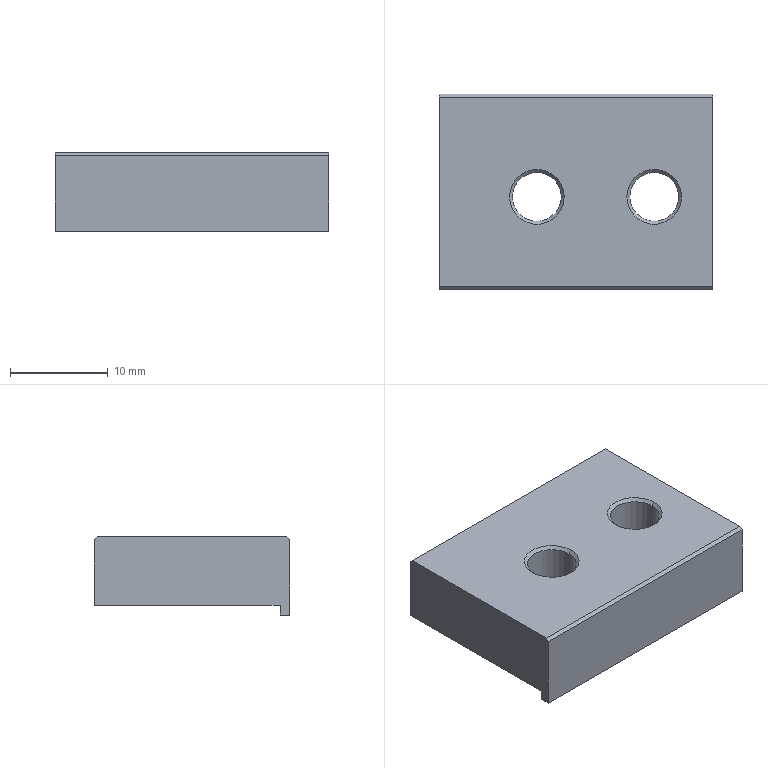Part | NX | 1 solid | 22 faces | box 28 x 20 x 8 mm | volume 3668 mm3 | plane 10 | cone 8 | cylinder 4 | commonest cylinder face diameters 5 x4
STEP:
#1=CARTESIAN_POINT('',(28.,0.7,7.));
#2=VERTEX_POINT('',#1);
#3=CARTESIAN_POINT('',(0.,0.7,7.));
#4=VERTEX_POINT('',#3);
#5=CARTESIAN_POINT('',(0.,0.7,7.));
#6=DIRECTION('',(-1.,0.,0.));
#7=VECTOR('',#6,1000.);
#8=LINE('',#5,#7);
#9=EDGE_CURVE('',#2,#4,#8,.T.);
#10=ORIENTED_EDGE('',*,*,#9,.T.);
#11=CARTESIAN_POINT('',(0.,-18.7,7.));
#12=VERTEX_POINT('',#11);
#13=CARTESIAN_POINT('',(0.,0.,7.));
#14=DIRECTION('',(0.,1.,0.));
#15=VECTOR('',#14,1000.);
#16=LINE('',#13,#15);
#17=EDGE_CURVE('',#12,#4,#16,.T.);
#18=ORIENTED_EDGE('',*,*,#17,.F.);
#19=CARTESIAN_POINT('',(28.,-18.7,7.));
#20=VERTEX_POINT('',#19);
#21=CARTESIAN_POINT('',(0.,-18.7,7.));
#22=DIRECTION('',(1.,0.,0.));
#23=VECTOR('',#22,1000.);
#24=LINE('',#21,#23);
#25=EDGE_CURVE('',#12,#20,#24,.T.);
#26=ORIENTED_EDGE('',*,*,#25,.T.);
#27=CARTESIAN_POINT('',(28.,0.,7.));
#28=DIRECTION('',(0.,-1.,0.));
#29=VECTOR('',#28,1000.);
#30=LINE('',#27,#29);
#31=EDGE_CURVE('',#2,#20,#30,.T.);
#32=ORIENTED_EDGE('',*,*,#31,.F.);
#33=EDGE_LOOP('',(#10,#18,#26,#32));
#34=FACE_BOUND('',#33,.T.);
#35=CARTESIAN_POINT('',(12.8,-9.5,7.));
#36=VERTEX_POINT('',#35);
#37=CARTESIAN_POINT('',(7.2,-9.5,7.));
#38=VERTEX_POINT('',#37);
#39=CARTESIAN_POINT('',(10.,-9.5,7.));
#40=DIRECTION('',(0.,0.,1.));
#41=DIRECTION('',(1.,0.,0.));
#42=AXIS2_PLACEMENT_3D('',#39,#40,#41);
#43=CIRCLE('',#42,2.8);
#44=EDGE_CURVE('',#36,#38,#43,.T.);
#45=ORIENTED_EDGE('',*,*,#44,.F.);
#46=CARTESIAN_POINT('',(10.,-9.5,7.));
#47=DIRECTION('',(0.,0.,1.));
#48=DIRECTION('',(1.,0.,0.));
#49=AXIS2_PLACEMENT_3D('',#46,#47,#48);
#50=CIRCLE('',#49,2.8);
#51=EDGE_CURVE('',#38,#36,#50,.T.);
#52=ORIENTED_EDGE('',*,*,#51,.F.);
#53=EDGE_LOOP('',(#45,#52));
#54=FACE_BOUND('',#53,.T.);
#55=CARTESIAN_POINT('',(19.2,-9.5,7.));
#56=VERTEX_POINT('',#55);
#57=CARTESIAN_POINT('',(24.8,-9.5,7.));
#58=VERTEX_POINT('',#57);
#59=CARTESIAN_POINT('',(22.,-9.5,7.));
#60=DIRECTION('',(0.,0.,1.));
#61=DIRECTION('',(1.,0.,0.));
#62=AXIS2_PLACEMENT_3D('',#59,#60,#61);
#63=CIRCLE('',#62,2.8);
#64=EDGE_CURVE('',#56,#58,#63,.T.);
#65=ORIENTED_EDGE('',*,*,#64,.F.);
#66=CARTESIAN_POINT('',(22.,-9.5,7.));
#67=DIRECTION('',(0.,0.,1.));
#68=DIRECTION('',(1.,0.,0.));
#69=AXIS2_PLACEMENT_3D('',#66,#67,#68);
#70=CIRCLE('',#69,2.8);
#71=EDGE_CURVE('',#58,#56,#70,.T.);
#72=ORIENTED_EDGE('',*,*,#71,.F.);
#73=EDGE_LOOP('',(#65,#72));
#74=FACE_BOUND('',#73,.T.);
#75=CARTESIAN_POINT('',(0.,0.,7.));
#76=DIRECTION('',(0.,0.,1.));
#77=DIRECTION('',(1.,0.,0.));
#78=AXIS2_PLACEMENT_3D('',#75,#76,#77);
#79=PLANE('',#78);
#80=ADVANCED_FACE('',(#34,#54,#74),#79,.T.);
#81=CARTESIAN_POINT('',(28.,1.,0.));
#82=VERTEX_POINT('',#81);
#83=CARTESIAN_POINT('',(28.,1.,6.7));
#84=VERTEX_POINT('',#83);
#85=CARTESIAN_POINT('',(28.,1.,0.));
#86=DIRECTION('',(0.,0.,1.));
#87=VECTOR('',#86,1000.);
#88=LINE('',#85,#87);
#89=EDGE_CURVE('',#82,#84,#88,.T.);
#90=ORIENTED_EDGE('',*,*,#89,.T.);
#91=CARTESIAN_POINT('',(28.,0.,7.7));
#92=DIRECTION('',(0.,-0.7071,0.7071));
#93=VECTOR('',#92,1000.);
#94=LINE('',#91,#93);
#95=EDGE_CURVE('',#84,#2,#94,.T.);
#96=ORIENTED_EDGE('',*,*,#95,.T.);
#97=ORIENTED_EDGE('',*,*,#31,.T.);
#98=CARTESIAN_POINT('',(28.,-19.,6.7));
#99=VERTEX_POINT('',#98);
#100=CARTESIAN_POINT('',(28.,0.,25.7));
#101=DIRECTION('',(0.,-0.7071,-0.7071));
#102=VECTOR('',#101,1000.);
#103=LINE('',#100,#102);
#104=EDGE_CURVE('',#20,#99,#103,.T.);
#105=ORIENTED_EDGE('',*,*,#104,.T.);
#106=CARTESIAN_POINT('',(28.,-19.,-1.));
#107=VERTEX_POINT('',#106);
#108=CARTESIAN_POINT('',(28.,-19.,0.));
#109=DIRECTION('',(0.,0.,-1.));
#110=VECTOR('',#109,1000.);
#111=LINE('',#108,#110);
#112=EDGE_CURVE('',#99,#107,#111,.T.);
#113=ORIENTED_EDGE('',*,*,#112,.T.);
#114=CARTESIAN_POINT('',(28.,-18.,-1.));
#115=VERTEX_POINT('',#114);
#116=CARTESIAN_POINT('',(28.,0.,-1.));
#117=DIRECTION('',(0.,1.,0.));
#118=VECTOR('',#117,1000.);
#119=LINE('',#116,#118);
#120=EDGE_CURVE('',#107,#115,#119,.T.);
#121=ORIENTED_EDGE('',*,*,#120,.T.);
#122=CARTESIAN_POINT('',(28.,-18.,0.));
#123=VERTEX_POINT('',#122);
#124=CARTESIAN_POINT('',(28.,-18.,0.));
#125=DIRECTION('',(0.,0.,-1.));
#126=VECTOR('',#125,1000.);
#127=LINE('',#124,#126);
#128=EDGE_CURVE('',#123,#115,#127,.T.);
#129=ORIENTED_EDGE('',*,*,#128,.F.);
#130=CARTESIAN_POINT('',(28.,0.,0.));
#131=DIRECTION('',(0.,-1.,0.));
#132=VECTOR('',#131,1000.);
#133=LINE('',#130,#132);
#134=EDGE_CURVE('',#82,#123,#133,.T.);
#135=ORIENTED_EDGE('',*,*,#134,.F.);
#136=EDGE_LOOP('',(#90,#96,#97,#105,#113,#121,#129,#135));
#137=FACE_BOUND('',#136,.T.);
#138=CARTESIAN_POINT('',(28.,-18.,0.));
#139=DIRECTION('',(1.,0.,0.));
#140=DIRECTION('',(0.,1.,0.));
#141=AXIS2_PLACEMENT_3D('',#138,#139,#140);
#142=PLANE('',#141);
#143=ADVANCED_FACE('',(#137),#142,.T.);
#144=CARTESIAN_POINT('',(0.,-18.,0.));
#145=VERTEX_POINT('',#144);
#146=CARTESIAN_POINT('',(0.,-18.,0.));
#147=DIRECTION('',(-1.,0.,0.));
#148=VECTOR('',#147,1000.);
#149=LINE('',#146,#148);
#150=EDGE_CURVE('',#123,#145,#149,.T.);
#151=ORIENTED_EDGE('',*,*,#150,.F.);
#152=ORIENTED_EDGE('',*,*,#128,.T.);
#153=CARTESIAN_POINT('',(0.,-18.,-1.));
#154=VERTEX_POINT('',#153);
#155=CARTESIAN_POINT('',(0.,-18.,-1.));
#156=DIRECTION('',(1.,0.,0.));
#157=VECTOR('',#156,1000.);
#158=LINE('',#155,#157);
#159=EDGE_CURVE('',#154,#115,#158,.T.);
#160=ORIENTED_EDGE('',*,*,#159,.F.);
#161=CARTESIAN_POINT('',(0.,-18.,0.));
#162=DIRECTION('',(0.,0.,1.));
#163=VECTOR('',#162,1000.);
#164=LINE('',#161,#163);
#165=EDGE_CURVE('',#154,#145,#164,.T.);
#166=ORIENTED_EDGE('',*,*,#165,.T.);
#167=EDGE_LOOP('',(#151,#152,#160,#166));
#168=FACE_BOUND('',#167,.T.);
#169=CARTESIAN_POINT('',(0.,-18.,0.));
#170=DIRECTION('',(0.,-1.,0.));
#171=DIRECTION('',(0.,0.,-1.));
#172=AXIS2_PLACEMENT_3D('',#169,#170,#171);
#173=PLANE('',#172);
#174=ADVANCED_FACE('',(#168),#173,.F.);
#175=CARTESIAN_POINT('',(0.,1.,0.));
#176=VERTEX_POINT('',#175);
#177=CARTESIAN_POINT('',(0.,0.,0.));
#178=DIRECTION('',(0.,1.,0.));
#179=VECTOR('',#178,1000.);
#180=LINE('',#177,#179);
#181=EDGE_CURVE('',#145,#176,#180,.T.);
#182=ORIENTED_EDGE('',*,*,#181,.F.);
#183=ORIENTED_EDGE('',*,*,#165,.F.);
#184=CARTESIAN_POINT('',(0.,-19.,-1.));
#185=VERTEX_POINT('',#184);
#186=CARTESIAN_POINT('',(0.,0.,-1.));
#187=DIRECTION('',(0.,-1.,0.));
#188=VECTOR('',#187,1000.);
#189=LINE('',#186,#188);
#190=EDGE_CURVE('',#154,#185,#189,.T.);
#191=ORIENTED_EDGE('',*,*,#190,.T.);
#192=CARTESIAN_POINT('',(0.,-19.,6.7));
#193=VERTEX_POINT('',#192);
#194=CARTESIAN_POINT('',(0.,-19.,0.));
#195=DIRECTION('',(0.,0.,1.));
#196=VECTOR('',#195,1000.);
#197=LINE('',#194,#196);
#198=EDGE_CURVE('',#185,#193,#197,.T.);
#199=ORIENTED_EDGE('',*,*,#198,.T.);
#200=CARTESIAN_POINT('',(0.,0.,25.7));
#201=DIRECTION('',(0.,0.7071,0.7071));
#202=VECTOR('',#201,1000.);
#203=LINE('',#200,#202);
#204=EDGE_CURVE('',#193,#12,#203,.T.);
#205=ORIENTED_EDGE('',*,*,#204,.T.);
#206=ORIENTED_EDGE('',*,*,#17,.T.);
#207=CARTESIAN_POINT('',(0.,1.,6.7));
#208=VERTEX_POINT('',#207);
#209=CARTESIAN_POINT('',(0.,0.,7.7));
#210=DIRECTION('',(0.,0.7071,-0.7071));
#211=VECTOR('',#210,1000.);
#212=LINE('',#209,#211);
#213=EDGE_CURVE('',#4,#208,#212,.T.);
#214=ORIENTED_EDGE('',*,*,#213,.T.);
#215=CARTESIAN_POINT('',(0.,1.,0.));
#216=DIRECTION('',(0.,0.,-1.));
#217=VECTOR('',#216,1000.);
#218=LINE('',#215,#217);
#219=EDGE_CURVE('',#208,#176,#218,.T.);
#220=ORIENTED_EDGE('',*,*,#219,.T.);
#221=EDGE_LOOP('',(#182,#183,#191,#199,#205,#206,#214,#220));
#222=FACE_BOUND('',#221,.T.);
#223=CARTESIAN_POINT('',(0.,0.,0.));
#224=DIRECTION('',(-1.,0.,0.));
#225=DIRECTION('',(0.,0.,1.));
#226=AXIS2_PLACEMENT_3D('',#223,#224,#225);
#227=PLANE('',#226);
#228=ADVANCED_FACE('',(#222),#227,.T.);
#229=CARTESIAN_POINT('',(0.,1.,0.));
#230=DIRECTION('',(1.,0.,0.));
#231=VECTOR('',#230,1000.);
#232=LINE('',#229,#231);
#233=EDGE_CURVE('',#176,#82,#232,.T.);
#234=ORIENTED_EDGE('',*,*,#233,.T.);
#235=ORIENTED_EDGE('',*,*,#134,.T.);
#236=ORIENTED_EDGE('',*,*,#150,.T.);
#237=ORIENTED_EDGE('',*,*,#181,.T.);
#238=EDGE_LOOP('',(#234,#235,#236,#237));
#239=FACE_BOUND('',#238,.T.);
#240=CARTESIAN_POINT('',(7.2,-9.5,0.));
#241=VERTEX_POINT('',#240);
#242=CARTESIAN_POINT('',(12.8,-9.5,0.));
#243=VERTEX_POINT('',#242);
#244=CARTESIAN_POINT('',(10.,-9.5,0.));
#245=DIRECTION('',(0.,0.,-1.));
#246=DIRECTION('',(-1.,0.,0.));
#247=AXIS2_PLACEMENT_3D('',#244,#245,#246);
#248=CIRCLE('',#247,2.8);
#249=EDGE_CURVE('',#241,#243,#248,.T.);
#250=ORIENTED_EDGE('',*,*,#249,.F.);
#251=CARTESIAN_POINT('',(10.,-9.5,0.));
#252=DIRECTION('',(0.,0.,-1.));
#253=DIRECTION('',(-1.,0.,0.));
#254=AXIS2_PLACEMENT_3D('',#251,#252,#253);
#255=CIRCLE('',#254,2.8);
#256=EDGE_CURVE('',#243,#241,#255,.T.);
#257=ORIENTED_EDGE('',*,*,#256,.F.);
#258=EDGE_LOOP('',(#250,#257));
#259=FACE_BOUND('',#258,.T.);
#260=CARTESIAN_POINT('',(19.2,-9.5,0.));
#261=VERTEX_POINT('',#260);
#262=CARTESIAN_POINT('',(24.8,-9.5,0.));
#263=VERTEX_POINT('',#262);
#264=CARTESIAN_POINT('',(22.,-9.5,0.));
#265=DIRECTION('',(0.,0.,-1.));
#266=DIRECTION('',(-1.,0.,0.));
#267=AXIS2_PLACEMENT_3D('',#264,#265,#266);
#268=CIRCLE('',#267,2.8);
#269=EDGE_CURVE('',#261,#263,#268,.T.);
#270=ORIENTED_EDGE('',*,*,#269,.F.);
#271=CARTESIAN_POINT('',(22.,-9.5,0.));
#272=DIRECTION('',(0.,0.,-1.));
#273=DIRECTION('',(-1.,0.,0.));
#274=AXIS2_PLACEMENT_3D('',#271,#272,#273);
#275=CIRCLE('',#274,2.8);
#276=EDGE_CURVE('',#263,#261,#275,.T.);
#277=ORIENTED_EDGE('',*,*,#276,.F.);
#278=EDGE_LOOP('',(#270,#277));
#279=FACE_BOUND('',#278,.T.);
#280=CARTESIAN_POINT('',(0.,0.,0.));
#281=DIRECTION('',(0.,0.,1.));
#282=DIRECTION('',(1.,0.,0.));
#283=AXIS2_PLACEMENT_3D('',#280,#281,#282);
#284=PLANE('',#283);
#285=ADVANCED_FACE('',(#239,#259,#279),#284,.F.);
#286=CARTESIAN_POINT('',(0.,-19.,6.7));
#287=DIRECTION('',(1.,0.,0.));
#288=VECTOR('',#287,1000.);
#289=LINE('',#286,#288);
#290=EDGE_CURVE('',#193,#99,#289,.T.);
#291=ORIENTED_EDGE('',*,*,#290,.F.);
#292=ORIENTED_EDGE('',*,*,#198,.F.);
#293=CARTESIAN_POINT('',(0.,-19.,-1.));
#294=DIRECTION('',(-1.,0.,0.));
#295=VECTOR('',#294,1000.);
#296=LINE('',#293,#295);
#297=EDGE_CURVE('',#107,#185,#296,.T.);
#298=ORIENTED_EDGE('',*,*,#297,.F.);
#299=ORIENTED_EDGE('',*,*,#112,.F.);
#300=EDGE_LOOP('',(#291,#292,#298,#299));
#301=FACE_BOUND('',#300,.T.);
#302=CARTESIAN_POINT('',(0.,-19.,0.));
#303=DIRECTION('',(0.,-1.,0.));
#304=DIRECTION('',(0.,0.,-1.));
#305=AXIS2_PLACEMENT_3D('',#302,#303,#304);
#306=PLANE('',#305);
#307=ADVANCED_FACE('',(#301),#306,.T.);
#308=ORIENTED_EDGE('',*,*,#159,.T.);
#309=ORIENTED_EDGE('',*,*,#120,.F.);
#310=ORIENTED_EDGE('',*,*,#297,.T.);
#311=ORIENTED_EDGE('',*,*,#190,.F.);
#312=EDGE_LOOP('',(#308,#309,#310,#311));
#313=FACE_BOUND('',#312,.T.);
#314=CARTESIAN_POINT('',(0.,-18.,-1.));
#315=DIRECTION('',(0.,0.,-1.));
#316=DIRECTION('',(0.,-1.,0.));
#317=AXIS2_PLACEMENT_3D('',#314,#315,#316);
#318=PLANE('',#317);
#319=ADVANCED_FACE('',(#313),#318,.T.);
#320=ORIENTED_EDGE('',*,*,#233,.F.);
#321=ORIENTED_EDGE('',*,*,#219,.F.);
#322=CARTESIAN_POINT('',(0.,1.,6.7));
#323=DIRECTION('',(1.,0.,0.));
#324=VECTOR('',#323,1000.);
#325=LINE('',#322,#324);
#326=EDGE_CURVE('',#208,#84,#325,.T.);
#327=ORIENTED_EDGE('',*,*,#326,.T.);
#328=ORIENTED_EDGE('',*,*,#89,.F.);
#329=EDGE_LOOP('',(#320,#321,#327,#328));
#330=FACE_BOUND('',#329,.T.);
#331=CARTESIAN_POINT('',(28.,1.,0.));
#332=DIRECTION('',(0.,1.,0.));
#333=DIRECTION('',(1.,0.,0.));
#334=AXIS2_PLACEMENT_3D('',#331,#332,#333);
#335=PLANE('',#334);
#336=ADVANCED_FACE('',(#330),#335,.T.);
#337=CARTESIAN_POINT('',(12.5,-9.5,0.3));
#338=VERTEX_POINT('',#337);
#339=CARTESIAN_POINT('',(7.5,-9.5,0.3));
#340=VERTEX_POINT('',#339);
#341=CARTESIAN_POINT('',(10.,-9.5,0.3));
#342=DIRECTION('',(0.,0.,-1.));
#343=DIRECTION('',(-1.,0.,0.));
#344=AXIS2_PLACEMENT_3D('',#341,#342,#343);
#345=CIRCLE('',#344,2.5);
#346=EDGE_CURVE('',#338,#340,#345,.T.);
#347=ORIENTED_EDGE('',*,*,#346,.T.);
#348=CARTESIAN_POINT('',(7.5,-9.5,6.7));
#349=VERTEX_POINT('',#348);
#350=CARTESIAN_POINT('',(7.5,-9.5,7.));
#351=DIRECTION('',(0.,0.,-1.));
#352=VECTOR('',#351,1000.);
#353=LINE('',#350,#352);
#354=EDGE_CURVE('',#340,#349,#353,.F.);
#355=ORIENTED_EDGE('',*,*,#354,.T.);
#356=CARTESIAN_POINT('',(12.5,-9.5,6.7));
#357=VERTEX_POINT('',#356);
#358=CARTESIAN_POINT('',(10.,-9.5,6.7));
#359=DIRECTION('',(0.,0.,1.));
#360=DIRECTION('',(1.,0.,0.));
#361=AXIS2_PLACEMENT_3D('',#358,#359,#360);
#362=CIRCLE('',#361,2.5);
#363=EDGE_CURVE('',#349,#357,#362,.T.);
#364=ORIENTED_EDGE('',*,*,#363,.T.);
#365=CARTESIAN_POINT('',(12.5,-9.5,7.));
#366=DIRECTION('',(0.,0.,-1.));
#367=VECTOR('',#366,1000.);
#368=LINE('',#365,#367);
#369=EDGE_CURVE('',#338,#357,#368,.F.);
#370=ORIENTED_EDGE('',*,*,#369,.F.);
#371=EDGE_LOOP('',(#347,#355,#364,#370));
#372=FACE_BOUND('',#371,.T.);
#373=CARTESIAN_POINT('',(10.,-9.5,7.));
#374=DIRECTION('',(0.,0.,-1.));
#375=DIRECTION('',(-1.,0.,0.));
#376=AXIS2_PLACEMENT_3D('',#373,#374,#375);
#377=CYLINDRICAL_SURFACE('',#376,2.5);
#378=ADVANCED_FACE('',(#372),#377,.F.);
#379=CARTESIAN_POINT('',(19.5,-9.5,6.7));
#380=VERTEX_POINT('',#379);
#381=CARTESIAN_POINT('',(24.5,-9.5,6.7));
#382=VERTEX_POINT('',#381);
#383=CARTESIAN_POINT('',(22.,-9.5,6.7));
#384=DIRECTION('',(0.,0.,1.));
#385=DIRECTION('',(1.,0.,0.));
#386=AXIS2_PLACEMENT_3D('',#383,#384,#385);
#387=CIRCLE('',#386,2.5);
#388=EDGE_CURVE('',#380,#382,#387,.T.);
#389=ORIENTED_EDGE('',*,*,#388,.T.);
#390=CARTESIAN_POINT('',(24.5,-9.5,0.3));
#391=VERTEX_POINT('',#390);
#392=CARTESIAN_POINT('',(24.5,-9.5,7.));
#393=DIRECTION('',(0.,0.,-1.));
#394=VECTOR('',#393,1000.);
#395=LINE('',#392,#394);
#396=EDGE_CURVE('',#382,#391,#395,.T.);
#397=ORIENTED_EDGE('',*,*,#396,.T.);
#398=CARTESIAN_POINT('',(19.5,-9.5,0.3));
#399=VERTEX_POINT('',#398);
#400=CARTESIAN_POINT('',(22.,-9.5,0.3));
#401=DIRECTION('',(0.,0.,-1.));
#402=DIRECTION('',(-1.,0.,0.));
#403=AXIS2_PLACEMENT_3D('',#400,#401,#402);
#404=CIRCLE('',#403,2.5);
#405=EDGE_CURVE('',#391,#399,#404,.T.);
#406=ORIENTED_EDGE('',*,*,#405,.T.);
#407=CARTESIAN_POINT('',(19.5,-9.5,7.));
#408=DIRECTION('',(0.,0.,-1.));
#409=VECTOR('',#408,1000.);
#410=LINE('',#407,#409);
#411=EDGE_CURVE('',#380,#399,#410,.T.);
#412=ORIENTED_EDGE('',*,*,#411,.F.);
#413=EDGE_LOOP('',(#389,#397,#406,#412));
#414=FACE_BOUND('',#413,.T.);
#415=CARTESIAN_POINT('',(22.,-9.5,7.));
#416=DIRECTION('',(0.,0.,-1.));
#417=DIRECTION('',(-1.,0.,0.));
#418=AXIS2_PLACEMENT_3D('',#415,#416,#417);
#419=CYLINDRICAL_SURFACE('',#418,2.5);
#420=ADVANCED_FACE('',(#414),#419,.F.);
#421=ORIENTED_EDGE('',*,*,#25,.F.);
#422=ORIENTED_EDGE('',*,*,#204,.F.);
#423=ORIENTED_EDGE('',*,*,#290,.T.);
#424=ORIENTED_EDGE('',*,*,#104,.F.);
#425=EDGE_LOOP('',(#421,#422,#423,#424));
#426=FACE_BOUND('',#425,.T.);
#427=CARTESIAN_POINT('',(14.,-18.85,6.85));
#428=DIRECTION('',(0.,-0.7071,0.7071));
#429=DIRECTION('',(-1.,0.,0.));
#430=AXIS2_PLACEMENT_3D('',#427,#428,#429);
#431=PLANE('',#430);
#432=ADVANCED_FACE('',(#426),#431,.T.);
#433=CARTESIAN_POINT('',(22.,-9.5,0.3));
#434=DIRECTION('',(0.,0.,-1.));
#435=DIRECTION('',(-1.,0.,0.));
#436=AXIS2_PLACEMENT_3D('',#433,#434,#435);
#437=CIRCLE('',#436,2.5);
#438=EDGE_CURVE('',#399,#391,#437,.T.);
#439=ORIENTED_EDGE('',*,*,#438,.F.);
#440=CARTESIAN_POINT('',(19.2,-9.5,0.));
#441=DIRECTION('',(-0.7071,0.,-0.7071));
#442=VECTOR('',#441,1000.);
#443=LINE('',#440,#442);
#444=EDGE_CURVE('',#261,#399,#443,.F.);
#445=ORIENTED_EDGE('',*,*,#444,.F.);
#446=ORIENTED_EDGE('',*,*,#269,.T.);
#447=CARTESIAN_POINT('',(24.8,-9.5,0.));
#448=DIRECTION('',(0.7071,0.,-0.7071));
#449=VECTOR('',#448,1000.);
#450=LINE('',#447,#449);
#451=EDGE_CURVE('',#263,#391,#450,.F.);
#452=ORIENTED_EDGE('',*,*,#451,.T.);
#453=EDGE_LOOP('',(#439,#445,#446,#452));
#454=FACE_BOUND('',#453,.T.);
#455=CARTESIAN_POINT('',(22.,-9.5,0.));
#456=DIRECTION('',(0.,0.,-1.));
#457=DIRECTION('',(-1.,0.,0.));
#458=AXIS2_PLACEMENT_3D('',#455,#456,#457);
#459=CONICAL_SURFACE('',#458,2.8,0.7854);
#460=ADVANCED_FACE('',(#454),#459,.F.);
#461=ORIENTED_EDGE('',*,*,#346,.F.);
#462=CARTESIAN_POINT('',(12.8,-9.5,0.));
#463=DIRECTION('',(0.7071,0.,-0.7071));
#464=VECTOR('',#463,1000.);
#465=LINE('',#462,#464);
#466=EDGE_CURVE('',#338,#243,#465,.T.);
#467=ORIENTED_EDGE('',*,*,#466,.T.);
#468=ORIENTED_EDGE('',*,*,#256,.T.);
#469=CARTESIAN_POINT('',(7.2,-9.5,0.));
#470=DIRECTION('',(-0.7071,0.,-0.7071));
#471=VECTOR('',#470,1000.);
#472=LINE('',#469,#471);
#473=EDGE_CURVE('',#340,#241,#472,.T.);
#474=ORIENTED_EDGE('',*,*,#473,.F.);
#475=EDGE_LOOP('',(#461,#467,#468,#474));
#476=FACE_BOUND('',#475,.T.);
#477=CARTESIAN_POINT('',(10.,-9.5,0.));
#478=DIRECTION('',(0.,0.,-1.));
#479=DIRECTION('',(-1.,0.,0.));
#480=AXIS2_PLACEMENT_3D('',#477,#478,#479);
#481=CONICAL_SURFACE('',#480,2.8,0.7854);
#482=ADVANCED_FACE('',(#476),#481,.F.);
#483=ORIENTED_EDGE('',*,*,#363,.F.);
#484=CARTESIAN_POINT('',(7.2,-9.5,7.));
#485=DIRECTION('',(-0.7071,0.,0.7071));
#486=VECTOR('',#485,1000.);
#487=LINE('',#484,#486);
#488=EDGE_CURVE('',#38,#349,#487,.F.);
#489=ORIENTED_EDGE('',*,*,#488,.F.);
#490=ORIENTED_EDGE('',*,*,#51,.T.);
#491=CARTESIAN_POINT('',(12.8,-9.5,7.));
#492=DIRECTION('',(0.7071,0.,0.7071));
#493=VECTOR('',#492,1000.);
#494=LINE('',#491,#493);
#495=EDGE_CURVE('',#36,#357,#494,.F.);
#496=ORIENTED_EDGE('',*,*,#495,.T.);
#497=EDGE_LOOP('',(#483,#489,#490,#496));
#498=FACE_BOUND('',#497,.T.);
#499=CARTESIAN_POINT('',(10.,-9.5,7.));
#500=DIRECTION('',(0.,0.,1.));
#501=DIRECTION('',(1.,0.,0.));
#502=AXIS2_PLACEMENT_3D('',#499,#500,#501);
#503=CONICAL_SURFACE('',#502,2.8,0.7854);
#504=ADVANCED_FACE('',(#498),#503,.F.);
#505=ORIENTED_EDGE('',*,*,#388,.F.);
#506=CARTESIAN_POINT('',(19.2,-9.5,7.));
#507=DIRECTION('',(-0.7071,0.,0.7071));
#508=VECTOR('',#507,1000.);
#509=LINE('',#506,#508);
#510=EDGE_CURVE('',#380,#56,#509,.T.);
#511=ORIENTED_EDGE('',*,*,#510,.T.);
#512=ORIENTED_EDGE('',*,*,#64,.T.);
#513=CARTESIAN_POINT('',(24.8,-9.5,7.));
#514=DIRECTION('',(0.7071,0.,0.7071));
#515=VECTOR('',#514,1000.);
#516=LINE('',#513,#515);
#517=EDGE_CURVE('',#382,#58,#516,.T.);
#518=ORIENTED_EDGE('',*,*,#517,.F.);
#519=EDGE_LOOP('',(#505,#511,#512,#518));
#520=FACE_BOUND('',#519,.T.);
#521=CARTESIAN_POINT('',(22.,-9.5,7.));
#522=DIRECTION('',(0.,0.,1.));
#523=DIRECTION('',(1.,0.,0.));
#524=AXIS2_PLACEMENT_3D('',#521,#522,#523);
#525=CONICAL_SURFACE('',#524,2.8,0.7854);
#526=ADVANCED_FACE('',(#520),#525,.F.);
#527=ORIENTED_EDGE('',*,*,#9,.F.);
#528=ORIENTED_EDGE('',*,*,#95,.F.);
#529=ORIENTED_EDGE('',*,*,#326,.F.);
#530=ORIENTED_EDGE('',*,*,#213,.F.);
#531=EDGE_LOOP('',(#527,#528,#529,#530));
#532=FACE_BOUND('',#531,.T.);
#533=CARTESIAN_POINT('',(14.,0.85,6.85));
#534=DIRECTION('',(0.,0.7071,0.7071));
#535=DIRECTION('',(1.,0.,0.));
#536=AXIS2_PLACEMENT_3D('',#533,#534,#535);
#537=PLANE('',#536);
#538=ADVANCED_FACE('',(#532),#537,.T.);
#539=ORIENTED_EDGE('',*,*,#438,.T.);
#540=ORIENTED_EDGE('',*,*,#396,.F.);
#541=CARTESIAN_POINT('',(22.,-9.5,6.7));
#542=DIRECTION('',(0.,0.,1.));
#543=DIRECTION('',(1.,0.,0.));
#544=AXIS2_PLACEMENT_3D('',#541,#542,#543);
#545=CIRCLE('',#544,2.5);
#546=EDGE_CURVE('',#382,#380,#545,.T.);
#547=ORIENTED_EDGE('',*,*,#546,.T.);
#548=ORIENTED_EDGE('',*,*,#411,.T.);
#549=EDGE_LOOP('',(#539,#540,#547,#548));
#550=FACE_BOUND('',#549,.T.);
#551=CARTESIAN_POINT('',(22.,-9.5,7.));
#552=DIRECTION('',(0.,0.,-1.));
#553=DIRECTION('',(-1.,0.,0.));
#554=AXIS2_PLACEMENT_3D('',#551,#552,#553);
#555=CYLINDRICAL_SURFACE('',#554,2.5);
#556=ADVANCED_FACE('',(#550),#555,.F.);
#557=ORIENTED_EDGE('',*,*,#354,.F.);
#558=CARTESIAN_POINT('',(10.,-9.5,0.3));
#559=DIRECTION('',(0.,0.,-1.));
#560=DIRECTION('',(-1.,0.,0.));
#561=AXIS2_PLACEMENT_3D('',#558,#559,#560);
#562=CIRCLE('',#561,2.5);
#563=EDGE_CURVE('',#340,#338,#562,.T.);
#564=ORIENTED_EDGE('',*,*,#563,.T.);
#565=ORIENTED_EDGE('',*,*,#369,.T.);
#566=CARTESIAN_POINT('',(10.,-9.5,6.7));
#567=DIRECTION('',(0.,0.,1.));
#568=DIRECTION('',(1.,0.,0.));
#569=AXIS2_PLACEMENT_3D('',#566,#567,#568);
#570=CIRCLE('',#569,2.5);
#571=EDGE_CURVE('',#357,#349,#570,.T.);
#572=ORIENTED_EDGE('',*,*,#571,.T.);
#573=EDGE_LOOP('',(#557,#564,#565,#572));
#574=FACE_BOUND('',#573,.T.);
#575=CARTESIAN_POINT('',(10.,-9.5,7.));
#576=DIRECTION('',(0.,0.,-1.));
#577=DIRECTION('',(-1.,0.,0.));
#578=AXIS2_PLACEMENT_3D('',#575,#576,#577);
#579=CYLINDRICAL_SURFACE('',#578,2.5);
#580=ADVANCED_FACE('',(#574),#579,.F.);
#581=ORIENTED_EDGE('',*,*,#517,.T.);
#582=ORIENTED_EDGE('',*,*,#71,.T.);
#583=ORIENTED_EDGE('',*,*,#510,.F.);
#584=ORIENTED_EDGE('',*,*,#546,.F.);
#585=EDGE_LOOP('',(#581,#582,#583,#584));
#586=FACE_BOUND('',#585,.T.);
#587=CARTESIAN_POINT('',(22.,-9.5,7.));
#588=DIRECTION('',(0.,0.,1.));
#589=DIRECTION('',(1.,0.,0.));
#590=AXIS2_PLACEMENT_3D('',#587,#588,#589);
#591=CONICAL_SURFACE('',#590,2.8,0.7854);
#592=ADVANCED_FACE('',(#586),#591,.F.);
#593=ORIENTED_EDGE('',*,*,#44,.T.);
#594=ORIENTED_EDGE('',*,*,#488,.T.);
#595=ORIENTED_EDGE('',*,*,#571,.F.);
#596=ORIENTED_EDGE('',*,*,#495,.F.);
#597=EDGE_LOOP('',(#593,#594,#595,#596));
#598=FACE_BOUND('',#597,.T.);
#599=CARTESIAN_POINT('',(10.,-9.5,7.));
#600=DIRECTION('',(0.,0.,1.));
#601=DIRECTION('',(1.,0.,0.));
#602=AXIS2_PLACEMENT_3D('',#599,#600,#601);
#603=CONICAL_SURFACE('',#602,2.8,0.7854);
#604=ADVANCED_FACE('',(#598),#603,.F.);
#605=ORIENTED_EDGE('',*,*,#444,.T.);
#606=ORIENTED_EDGE('',*,*,#405,.F.);
#607=ORIENTED_EDGE('',*,*,#451,.F.);
#608=ORIENTED_EDGE('',*,*,#276,.T.);
#609=EDGE_LOOP('',(#605,#606,#607,#608));
#610=FACE_BOUND('',#609,.T.);
#611=CARTESIAN_POINT('',(22.,-9.5,0.));
#612=DIRECTION('',(0.,0.,-1.));
#613=DIRECTION('',(-1.,0.,0.));
#614=AXIS2_PLACEMENT_3D('',#611,#612,#613);
#615=CONICAL_SURFACE('',#614,2.8,0.7854);
#616=ADVANCED_FACE('',(#610),#615,.F.);
#617=ORIENTED_EDGE('',*,*,#249,.T.);
#618=ORIENTED_EDGE('',*,*,#466,.F.);
#619=ORIENTED_EDGE('',*,*,#563,.F.);
#620=ORIENTED_EDGE('',*,*,#473,.T.);
#621=EDGE_LOOP('',(#617,#618,#619,#620));
#622=FACE_BOUND('',#621,.T.);
#623=CARTESIAN_POINT('',(10.,-9.5,0.));
#624=DIRECTION('',(0.,0.,-1.));
#625=DIRECTION('',(-1.,0.,0.));
#626=AXIS2_PLACEMENT_3D('',#623,#624,#625);
#627=CONICAL_SURFACE('',#626,2.8,0.7854);
#628=ADVANCED_FACE('',(#622),#627,.F.);
#629=CLOSED_SHELL('',(#80,#143,#174,#228,#285,#307,#319,#336,#378,#420,#432,#460,#482,#504,#526,#538,#556,#580,#592,#604,#616,#628));
#630=MANIFOLD_SOLID_BREP('',#629);
#631=(LENGTH_UNIT()NAMED_UNIT(*)SI_UNIT(.MILLI.,.METRE.));
#632=UNCERTAINTY_MEASURE_WITH_UNIT(LENGTH_MEASURE(0.00001),#631,'','');
#633=(NAMED_UNIT(*)PLANE_ANGLE_UNIT()SI_UNIT($,.RADIAN.));
#634=(NAMED_UNIT(*)SI_UNIT($,.STERADIAN.)SOLID_ANGLE_UNIT());
#635=(GEOMETRIC_REPRESENTATION_CONTEXT(3)GLOBAL_UNCERTAINTY_ASSIGNED_CONTEXT((#632))GLOBAL_UNIT_ASSIGNED_CONTEXT((#631,#633,#634))REPRESENTATION_CONTEXT('',''));
#636=ADVANCED_BREP_SHAPE_REPRESENTATION('',(#630),#635);